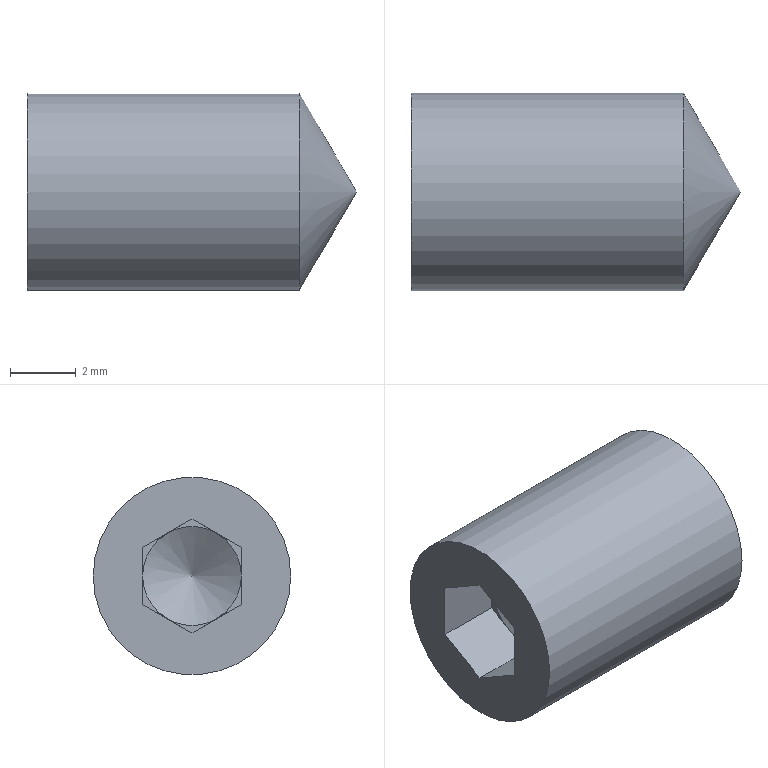Part | NX | features DATUM_CSYS 4, SKETCH 3, SWP104 2, EXTRUDE 1 | 1 solid | 16 faces | box 10 x 6 x 6 mm | volume 232.466 mm3 | plane 13 | cone 2 | cylinder 1 | commonest cylinder face diameters 6 x1
STEP:
#1=CARTESIAN_POINT('',(2.,1.5,0.));
#2=VERTEX_POINT('',#1);
#3=CARTESIAN_POINT('',(2.,1.5,0.866));
#4=VERTEX_POINT('',#3);
#5=CARTESIAN_POINT('',(2.,1.5,0.866));
#6=DIRECTION('',(0.,0.,-1.));
#7=VECTOR('',#6,1000.);
#8=LINE('',#5,#7);
#9=EDGE_CURVE('',#2,#4,#8,.F.);
#10=ORIENTED_EDGE('',*,*,#9,.F.);
#11=CARTESIAN_POINT('',(2.,0.75,1.299));
#12=VERTEX_POINT('',#11);
#13=CARTESIAN_POINT('',(2.,0.,0.));
#14=DIRECTION('',(1.,0.,0.));
#15=DIRECTION('',(0.,1.,0.));
#16=AXIS2_PLACEMENT_3D('',#13,#14,#15);
#17=CIRCLE('',#16,1.5);
#18=EDGE_CURVE('',#2,#12,#17,.T.);
#19=ORIENTED_EDGE('',*,*,#18,.T.);
#20=CARTESIAN_POINT('',(2.,0.,1.732));
#21=DIRECTION('',(0.,0.866,-0.5));
#22=VECTOR('',#21,1000.);
#23=LINE('',#20,#22);
#24=EDGE_CURVE('',#4,#12,#23,.F.);
#25=ORIENTED_EDGE('',*,*,#24,.F.);
#26=EDGE_LOOP('',(#10,#19,#25));
#27=FACE_BOUND('',#26,.T.);
#28=CARTESIAN_POINT('',(2.,0.,0.));
#29=DIRECTION('',(-1.,0.,0.));
#30=DIRECTION('',(0.,-1.,0.));
#31=AXIS2_PLACEMENT_3D('',#28,#29,#30);
#32=PLANE('',#31);
#33=ADVANCED_FACE('',(#27),#32,.T.);
#34=CARTESIAN_POINT('',(2.,0.,1.732));
#35=VERTEX_POINT('',#34);
#36=CARTESIAN_POINT('',(2.,0.,1.732));
#37=DIRECTION('',(0.,0.866,-0.5));
#38=VECTOR('',#37,1000.);
#39=LINE('',#36,#38);
#40=EDGE_CURVE('',#12,#35,#39,.F.);
#41=ORIENTED_EDGE('',*,*,#40,.F.);
#42=CARTESIAN_POINT('',(2.,-0.75,1.299));
#43=VERTEX_POINT('',#42);
#44=CARTESIAN_POINT('',(2.,0.,0.));
#45=DIRECTION('',(1.,0.,0.));
#46=DIRECTION('',(0.,1.,0.));
#47=AXIS2_PLACEMENT_3D('',#44,#45,#46);
#48=CIRCLE('',#47,1.5);
#49=EDGE_CURVE('',#12,#43,#48,.T.);
#50=ORIENTED_EDGE('',*,*,#49,.T.);
#51=CARTESIAN_POINT('',(2.,-1.5,0.866));
#52=DIRECTION('',(0.,0.866,0.5));
#53=VECTOR('',#52,1000.);
#54=LINE('',#51,#53);
#55=EDGE_CURVE('',#35,#43,#54,.F.);
#56=ORIENTED_EDGE('',*,*,#55,.F.);
#57=EDGE_LOOP('',(#41,#50,#56));
#58=FACE_BOUND('',#57,.T.);
#59=CARTESIAN_POINT('',(2.,0.,0.));
#60=DIRECTION('',(-1.,0.,0.));
#61=DIRECTION('',(0.,-1.,0.));
#62=AXIS2_PLACEMENT_3D('',#59,#60,#61);
#63=PLANE('',#62);
#64=ADVANCED_FACE('',(#58),#63,.T.);
#65=CARTESIAN_POINT('',(2.,-1.5,0.866));
#66=VERTEX_POINT('',#65);
#67=CARTESIAN_POINT('',(2.,-1.5,0.866));
#68=DIRECTION('',(0.,0.866,0.5));
#69=VECTOR('',#68,1000.);
#70=LINE('',#67,#69);
#71=EDGE_CURVE('',#43,#66,#70,.F.);
#72=ORIENTED_EDGE('',*,*,#71,.F.);
#73=CARTESIAN_POINT('',(2.,-1.5,0.));
#74=VERTEX_POINT('',#73);
#75=CARTESIAN_POINT('',(2.,0.,0.));
#76=DIRECTION('',(1.,0.,0.));
#77=DIRECTION('',(0.,1.,0.));
#78=AXIS2_PLACEMENT_3D('',#75,#76,#77);
#79=CIRCLE('',#78,1.5);
#80=EDGE_CURVE('',#43,#74,#79,.T.);
#81=ORIENTED_EDGE('',*,*,#80,.T.);
#82=CARTESIAN_POINT('',(2.,-1.5,-0.866));
#83=DIRECTION('',(0.,0.,1.));
#84=VECTOR('',#83,1000.);
#85=LINE('',#82,#84);
#86=EDGE_CURVE('',#66,#74,#85,.F.);
#87=ORIENTED_EDGE('',*,*,#86,.F.);
#88=EDGE_LOOP('',(#72,#81,#87));
#89=FACE_BOUND('',#88,.T.);
#90=CARTESIAN_POINT('',(2.,0.,0.));
#91=DIRECTION('',(-1.,0.,0.));
#92=DIRECTION('',(0.,-1.,0.));
#93=AXIS2_PLACEMENT_3D('',#90,#91,#92);
#94=PLANE('',#93);
#95=ADVANCED_FACE('',(#89),#94,.T.);
#96=CARTESIAN_POINT('',(2.,-1.5,-0.866));
#97=VERTEX_POINT('',#96);
#98=CARTESIAN_POINT('',(2.,-1.5,-0.866));
#99=DIRECTION('',(0.,0.,1.));
#100=VECTOR('',#99,1000.);
#101=LINE('',#98,#100);
#102=EDGE_CURVE('',#74,#97,#101,.F.);
#103=ORIENTED_EDGE('',*,*,#102,.F.);
#104=CARTESIAN_POINT('',(2.,-0.75,-1.299));
#105=VERTEX_POINT('',#104);
#106=CARTESIAN_POINT('',(2.,0.,0.));
#107=DIRECTION('',(1.,0.,0.));
#108=DIRECTION('',(0.,1.,0.));
#109=AXIS2_PLACEMENT_3D('',#106,#107,#108);
#110=CIRCLE('',#109,1.5);
#111=EDGE_CURVE('',#74,#105,#110,.T.);
#112=ORIENTED_EDGE('',*,*,#111,.T.);
#113=CARTESIAN_POINT('',(2.,0.,-1.732));
#114=DIRECTION('',(0.,-0.866,0.5));
#115=VECTOR('',#114,1000.);
#116=LINE('',#113,#115);
#117=EDGE_CURVE('',#97,#105,#116,.F.);
#118=ORIENTED_EDGE('',*,*,#117,.F.);
#119=EDGE_LOOP('',(#103,#112,#118));
#120=FACE_BOUND('',#119,.T.);
#121=CARTESIAN_POINT('',(2.,0.,0.));
#122=DIRECTION('',(-1.,0.,0.));
#123=DIRECTION('',(0.,-1.,0.));
#124=AXIS2_PLACEMENT_3D('',#121,#122,#123);
#125=PLANE('',#124);
#126=ADVANCED_FACE('',(#120),#125,.T.);
#127=CARTESIAN_POINT('',(2.,0.,-1.732));
#128=VERTEX_POINT('',#127);
#129=CARTESIAN_POINT('',(2.,0.,-1.732));
#130=DIRECTION('',(0.,-0.866,0.5));
#131=VECTOR('',#130,1000.);
#132=LINE('',#129,#131);
#133=EDGE_CURVE('',#105,#128,#132,.F.);
#134=ORIENTED_EDGE('',*,*,#133,.F.);
#135=CARTESIAN_POINT('',(2.,0.75,-1.299));
#136=VERTEX_POINT('',#135);
#137=CARTESIAN_POINT('',(2.,0.,0.));
#138=DIRECTION('',(1.,0.,0.));
#139=DIRECTION('',(0.,1.,0.));
#140=AXIS2_PLACEMENT_3D('',#137,#138,#139);
#141=CIRCLE('',#140,1.5);
#142=EDGE_CURVE('',#105,#136,#141,.T.);
#143=ORIENTED_EDGE('',*,*,#142,.T.);
#144=CARTESIAN_POINT('',(2.,1.5,-0.866));
#145=DIRECTION('',(0.,-0.866,-0.5));
#146=VECTOR('',#145,1000.);
#147=LINE('',#144,#146);
#148=EDGE_CURVE('',#128,#136,#147,.F.);
#149=ORIENTED_EDGE('',*,*,#148,.F.);
#150=EDGE_LOOP('',(#134,#143,#149));
#151=FACE_BOUND('',#150,.T.);
#152=CARTESIAN_POINT('',(2.,0.,0.));
#153=DIRECTION('',(-1.,0.,0.));
#154=DIRECTION('',(0.,-1.,0.));
#155=AXIS2_PLACEMENT_3D('',#152,#153,#154);
#156=PLANE('',#155);
#157=ADVANCED_FACE('',(#151),#156,.T.);
#158=CARTESIAN_POINT('',(8.268,3.,0.));
#159=VERTEX_POINT('',#158);
#160=CARTESIAN_POINT('',(8.268,0.,0.));
#161=DIRECTION('',(1.,0.,0.));
#162=DIRECTION('',(0.,1.,0.));
#163=AXIS2_PLACEMENT_3D('',#160,#161,#162);
#164=CIRCLE('',#163,3.);
#165=EDGE_CURVE('',#159,#159,#164,.T.);
#166=ORIENTED_EDGE('',*,*,#165,.F.);
#167=EDGE_LOOP('',(#166));
#168=FACE_BOUND('',#167,.T.);
#169=CARTESIAN_POINT('',(0.,3.,0.));
#170=VERTEX_POINT('',#169);
#171=CARTESIAN_POINT('',(0.,0.,0.));
#172=DIRECTION('',(1.,0.,0.));
#173=DIRECTION('',(0.,1.,0.));
#174=AXIS2_PLACEMENT_3D('',#171,#172,#173);
#175=CIRCLE('',#174,3.);
#176=EDGE_CURVE('',#170,#170,#175,.T.);
#177=ORIENTED_EDGE('',*,*,#176,.T.);
#178=EDGE_LOOP('',(#177));
#179=FACE_BOUND('',#178,.T.);
#180=CARTESIAN_POINT('',(0.,0.,0.));
#181=DIRECTION('',(1.,0.,0.));
#182=DIRECTION('',(0.,1.,0.));
#183=AXIS2_PLACEMENT_3D('',#180,#181,#182);
#184=CYLINDRICAL_SURFACE('',#183,3.);
#185=ADVANCED_FACE('',(#168,#179),#184,.T.);
#186=CARTESIAN_POINT('',(10.,0.,0.));
#187=VERTEX_POINT('',#186);
#188=VERTEX_LOOP('',#187);
#189=FACE_BOUND('',#188,.T.);
#190=ORIENTED_EDGE('',*,*,#165,.T.);
#191=EDGE_LOOP('',(#190));
#192=FACE_BOUND('',#191,.T.);
#193=CARTESIAN_POINT('',(8.268,0.,0.));
#194=DIRECTION('',(-1.,0.,0.));
#195=DIRECTION('',(0.,-1.,0.));
#196=AXIS2_PLACEMENT_3D('',#193,#194,#195);
#197=CONICAL_SURFACE('',#196,3.,1.047);
#198=ADVANCED_FACE('',(#189,#192),#197,.T.);
#199=CARTESIAN_POINT('',(0.,-1.5,0.866));
#200=VERTEX_POINT('',#199);
#201=CARTESIAN_POINT('',(0.,0.,1.732));
#202=VERTEX_POINT('',#201);
#203=CARTESIAN_POINT('',(0.,-1.5,0.866));
#204=DIRECTION('',(0.,0.866,0.5));
#205=VECTOR('',#204,1000.);
#206=LINE('',#203,#205);
#207=EDGE_CURVE('',#200,#202,#206,.T.);
#208=ORIENTED_EDGE('',*,*,#207,.F.);
#209=CARTESIAN_POINT('',(0.,-1.5,-0.866));
#210=VERTEX_POINT('',#209);
#211=CARTESIAN_POINT('',(0.,-1.5,-0.866));
#212=DIRECTION('',(0.,0.,1.));
#213=VECTOR('',#212,1000.);
#214=LINE('',#211,#213);
#215=EDGE_CURVE('',#210,#200,#214,.T.);
#216=ORIENTED_EDGE('',*,*,#215,.F.);
#217=CARTESIAN_POINT('',(0.,0.,-1.732));
#218=VERTEX_POINT('',#217);
#219=CARTESIAN_POINT('',(0.,0.,-1.732));
#220=DIRECTION('',(0.,-0.866,0.5));
#221=VECTOR('',#220,1000.);
#222=LINE('',#219,#221);
#223=EDGE_CURVE('',#218,#210,#222,.T.);
#224=ORIENTED_EDGE('',*,*,#223,.F.);
#225=CARTESIAN_POINT('',(0.,1.5,-0.866));
#226=VERTEX_POINT('',#225);
#227=CARTESIAN_POINT('',(0.,1.5,-0.866));
#228=DIRECTION('',(0.,-0.866,-0.5));
#229=VECTOR('',#228,1000.);
#230=LINE('',#227,#229);
#231=EDGE_CURVE('',#226,#218,#230,.T.);
#232=ORIENTED_EDGE('',*,*,#231,.F.);
#233=CARTESIAN_POINT('',(0.,1.5,0.866));
#234=VERTEX_POINT('',#233);
#235=CARTESIAN_POINT('',(0.,1.5,0.866));
#236=DIRECTION('',(0.,0.,-1.));
#237=VECTOR('',#236,1000.);
#238=LINE('',#235,#237);
#239=EDGE_CURVE('',#234,#226,#238,.T.);
#240=ORIENTED_EDGE('',*,*,#239,.F.);
#241=CARTESIAN_POINT('',(0.,0.,1.732));
#242=DIRECTION('',(0.,0.866,-0.5));
#243=VECTOR('',#242,1000.);
#244=LINE('',#241,#243);
#245=EDGE_CURVE('',#202,#234,#244,.T.);
#246=ORIENTED_EDGE('',*,*,#245,.F.);
#247=EDGE_LOOP('',(#208,#216,#224,#232,#240,#246));
#248=FACE_BOUND('',#247,.T.);
#249=ORIENTED_EDGE('',*,*,#176,.F.);
#250=EDGE_LOOP('',(#249));
#251=FACE_BOUND('',#250,.T.);
#252=CARTESIAN_POINT('',(0.,0.,0.));
#253=DIRECTION('',(1.,0.,0.));
#254=DIRECTION('',(0.,1.,0.));
#255=AXIS2_PLACEMENT_3D('',#252,#253,#254);
#256=PLANE('',#255);
#257=ADVANCED_FACE('',(#248,#251),#256,.F.);
#258=ORIENTED_EDGE('',*,*,#215,.T.);
#259=CARTESIAN_POINT('',(2.,-1.5,0.866));
#260=DIRECTION('',(-1.,0.,0.));
#261=VECTOR('',#260,1000.);
#262=LINE('',#259,#261);
#263=EDGE_CURVE('',#200,#66,#262,.F.);
#264=ORIENTED_EDGE('',*,*,#263,.T.);
#265=ORIENTED_EDGE('',*,*,#86,.T.);
#266=ORIENTED_EDGE('',*,*,#102,.T.);
#267=CARTESIAN_POINT('',(2.,-1.5,-0.866));
#268=DIRECTION('',(-1.,0.,0.));
#269=VECTOR('',#268,1000.);
#270=LINE('',#267,#269);
#271=EDGE_CURVE('',#210,#97,#270,.F.);
#272=ORIENTED_EDGE('',*,*,#271,.F.);
#273=EDGE_LOOP('',(#258,#264,#265,#266,#272));
#274=FACE_BOUND('',#273,.T.);
#275=CARTESIAN_POINT('',(2.,-1.5,-0.866));
#276=DIRECTION('',(0.,-1.,0.));
#277=DIRECTION('',(1.,0.,0.));
#278=AXIS2_PLACEMENT_3D('',#275,#276,#277);
#279=PLANE('',#278);
#280=ADVANCED_FACE('',(#274),#279,.F.);
#281=ORIENTED_EDGE('',*,*,#207,.T.);
#282=CARTESIAN_POINT('',(2.,0.,1.732));
#283=DIRECTION('',(-1.,0.,0.));
#284=VECTOR('',#283,1000.);
#285=LINE('',#282,#284);
#286=EDGE_CURVE('',#202,#35,#285,.F.);
#287=ORIENTED_EDGE('',*,*,#286,.T.);
#288=ORIENTED_EDGE('',*,*,#55,.T.);
#289=ORIENTED_EDGE('',*,*,#71,.T.);
#290=ORIENTED_EDGE('',*,*,#263,.F.);
#291=EDGE_LOOP('',(#281,#287,#288,#289,#290));
#292=FACE_BOUND('',#291,.T.);
#293=CARTESIAN_POINT('',(2.,-1.5,0.866));
#294=DIRECTION('',(0.,-0.5,0.866));
#295=DIRECTION('',(0.,-0.866,-0.5));
#296=AXIS2_PLACEMENT_3D('',#293,#294,#295);
#297=PLANE('',#296);
#298=ADVANCED_FACE('',(#292),#297,.F.);
#299=ORIENTED_EDGE('',*,*,#245,.T.);
#300=CARTESIAN_POINT('',(2.,1.5,0.866));
#301=DIRECTION('',(-1.,0.,0.));
#302=VECTOR('',#301,1000.);
#303=LINE('',#300,#302);
#304=EDGE_CURVE('',#234,#4,#303,.F.);
#305=ORIENTED_EDGE('',*,*,#304,.T.);
#306=ORIENTED_EDGE('',*,*,#24,.T.);
#307=ORIENTED_EDGE('',*,*,#40,.T.);
#308=ORIENTED_EDGE('',*,*,#286,.F.);
#309=EDGE_LOOP('',(#299,#305,#306,#307,#308));
#310=FACE_BOUND('',#309,.T.);
#311=CARTESIAN_POINT('',(2.,0.,1.732));
#312=DIRECTION('',(0.,0.5,0.866));
#313=DIRECTION('',(0.,-0.866,0.5));
#314=AXIS2_PLACEMENT_3D('',#311,#312,#313);
#315=PLANE('',#314);
#316=ADVANCED_FACE('',(#310),#315,.F.);
#317=ORIENTED_EDGE('',*,*,#239,.T.);
#318=CARTESIAN_POINT('',(2.,1.5,-0.866));
#319=VERTEX_POINT('',#318);
#320=CARTESIAN_POINT('',(2.,1.5,-0.866));
#321=DIRECTION('',(-1.,0.,0.));
#322=VECTOR('',#321,1000.);
#323=LINE('',#320,#322);
#324=EDGE_CURVE('',#226,#319,#323,.F.);
#325=ORIENTED_EDGE('',*,*,#324,.T.);
#326=CARTESIAN_POINT('',(2.,1.5,0.866));
#327=DIRECTION('',(0.,0.,-1.));
#328=VECTOR('',#327,1000.);
#329=LINE('',#326,#328);
#330=EDGE_CURVE('',#319,#2,#329,.F.);
#331=ORIENTED_EDGE('',*,*,#330,.T.);
#332=ORIENTED_EDGE('',*,*,#9,.T.);
#333=ORIENTED_EDGE('',*,*,#304,.F.);
#334=EDGE_LOOP('',(#317,#325,#331,#332,#333));
#335=FACE_BOUND('',#334,.T.);
#336=CARTESIAN_POINT('',(2.,1.5,0.866));
#337=DIRECTION('',(0.,1.,0.));
#338=DIRECTION('',(-1.,0.,0.));
#339=AXIS2_PLACEMENT_3D('',#336,#337,#338);
#340=PLANE('',#339);
#341=ADVANCED_FACE('',(#335),#340,.F.);
#342=ORIENTED_EDGE('',*,*,#231,.T.);
#343=CARTESIAN_POINT('',(2.,0.,-1.732));
#344=DIRECTION('',(-1.,0.,0.));
#345=VECTOR('',#344,1000.);
#346=LINE('',#343,#345);
#347=EDGE_CURVE('',#218,#128,#346,.F.);
#348=ORIENTED_EDGE('',*,*,#347,.T.);
#349=ORIENTED_EDGE('',*,*,#148,.T.);
#350=CARTESIAN_POINT('',(2.,1.5,-0.866));
#351=DIRECTION('',(0.,-0.866,-0.5));
#352=VECTOR('',#351,1000.);
#353=LINE('',#350,#352);
#354=EDGE_CURVE('',#136,#319,#353,.F.);
#355=ORIENTED_EDGE('',*,*,#354,.T.);
#356=ORIENTED_EDGE('',*,*,#324,.F.);
#357=EDGE_LOOP('',(#342,#348,#349,#355,#356));
#358=FACE_BOUND('',#357,.T.);
#359=CARTESIAN_POINT('',(2.,1.5,-0.866));
#360=DIRECTION('',(0.,0.5,-0.866));
#361=DIRECTION('',(0.,0.866,0.5));
#362=AXIS2_PLACEMENT_3D('',#359,#360,#361);
#363=PLANE('',#362);
#364=ADVANCED_FACE('',(#358),#363,.F.);
#365=ORIENTED_EDGE('',*,*,#223,.T.);
#366=ORIENTED_EDGE('',*,*,#271,.T.);
#367=ORIENTED_EDGE('',*,*,#117,.T.);
#368=ORIENTED_EDGE('',*,*,#133,.T.);
#369=ORIENTED_EDGE('',*,*,#347,.F.);
#370=EDGE_LOOP('',(#365,#366,#367,#368,#369));
#371=FACE_BOUND('',#370,.T.);
#372=CARTESIAN_POINT('',(2.,0.,-1.732));
#373=DIRECTION('',(0.,-0.5,-0.866));
#374=DIRECTION('',(0.,0.866,-0.5));
#375=AXIS2_PLACEMENT_3D('',#372,#373,#374);
#376=PLANE('',#375);
#377=ADVANCED_FACE('',(#371),#376,.F.);
#378=ORIENTED_EDGE('',*,*,#354,.F.);
#379=CARTESIAN_POINT('',(2.,0.,0.));
#380=DIRECTION('',(1.,0.,0.));
#381=DIRECTION('',(0.,1.,0.));
#382=AXIS2_PLACEMENT_3D('',#379,#380,#381);
#383=CIRCLE('',#382,1.5);
#384=EDGE_CURVE('',#136,#2,#383,.T.);
#385=ORIENTED_EDGE('',*,*,#384,.T.);
#386=ORIENTED_EDGE('',*,*,#330,.F.);
#387=EDGE_LOOP('',(#378,#385,#386));
#388=FACE_BOUND('',#387,.T.);
#389=CARTESIAN_POINT('',(2.,0.,0.));
#390=DIRECTION('',(-1.,0.,0.));
#391=DIRECTION('',(0.,-1.,0.));
#392=AXIS2_PLACEMENT_3D('',#389,#390,#391);
#393=PLANE('',#392);
#394=ADVANCED_FACE('',(#388),#393,.T.);
#395=ORIENTED_EDGE('',*,*,#18,.F.);
#396=ORIENTED_EDGE('',*,*,#384,.F.);
#397=ORIENTED_EDGE('',*,*,#142,.F.);
#398=ORIENTED_EDGE('',*,*,#111,.F.);
#399=ORIENTED_EDGE('',*,*,#80,.F.);
#400=ORIENTED_EDGE('',*,*,#49,.F.);
#401=EDGE_LOOP('',(#395,#396,#397,#398,#399,#400));
#402=FACE_BOUND('',#401,.T.);
#403=CARTESIAN_POINT('',(2.866,0.,0.));
#404=VERTEX_POINT('',#403);
#405=VERTEX_LOOP('',#404);
#406=FACE_BOUND('',#405,.T.);
#407=CARTESIAN_POINT('',(2.866,0.,0.));
#408=DIRECTION('',(-1.,0.,0.));
#409=DIRECTION('',(0.,-1.,0.));
#410=AXIS2_PLACEMENT_3D('',#407,#408,#409);
#411=CONICAL_SURFACE('',#410,0.,1.047);
#412=ADVANCED_FACE('',(#402,#406),#411,.F.);
#413=CLOSED_SHELL('',(#33,#64,#95,#126,#157,#185,#198,#257,#280,#298,#316,#341,#364,#377,#394,#412));
#414=MANIFOLD_SOLID_BREP('',#413);
#415=(LENGTH_UNIT()NAMED_UNIT(*)SI_UNIT(.MILLI.,.METRE.));
#416=UNCERTAINTY_MEASURE_WITH_UNIT(LENGTH_MEASURE(0.00001),#415,'','');
#417=(NAMED_UNIT(*)PLANE_ANGLE_UNIT()SI_UNIT($,.RADIAN.));
#418=(NAMED_UNIT(*)SI_UNIT($,.STERADIAN.)SOLID_ANGLE_UNIT());
#419=(GEOMETRIC_REPRESENTATION_CONTEXT(3)GLOBAL_UNCERTAINTY_ASSIGNED_CONTEXT((#416))GLOBAL_UNIT_ASSIGNED_CONTEXT((#415,#417,#418))REPRESENTATION_CONTEXT('',''));
#420=ADVANCED_BREP_SHAPE_REPRESENTATION('',(#414),#419);